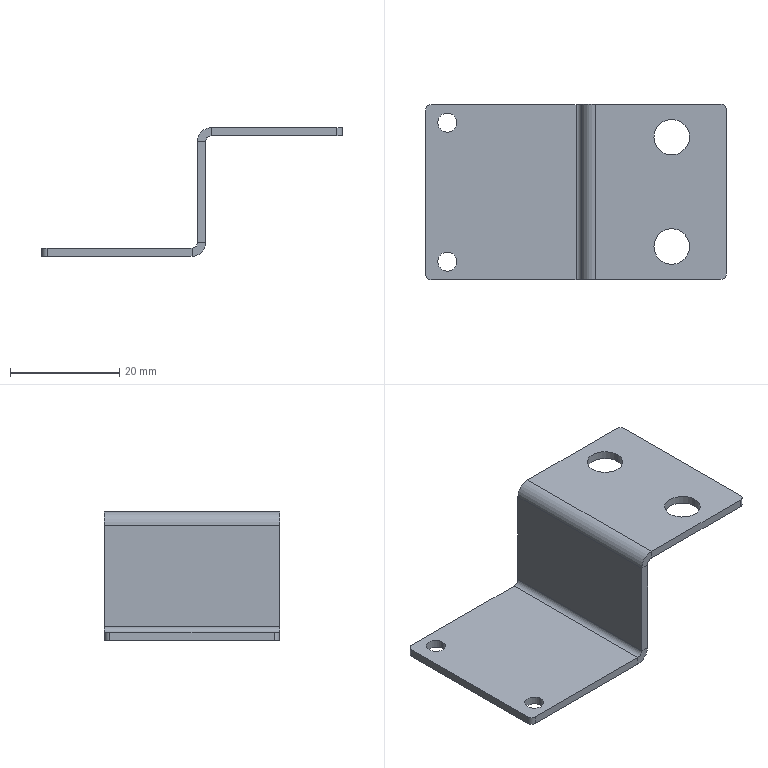Part | STEP file | Photoelectric adapter plate 4 | 1 solid | 34 faces | box 55 x 32 x 23.5 mm | volume 3494 mm3 | plane 18 | cylinder 16 | commonest cylinder face diameters 2 x6 3.5 x4 6.5 x4 5 x2